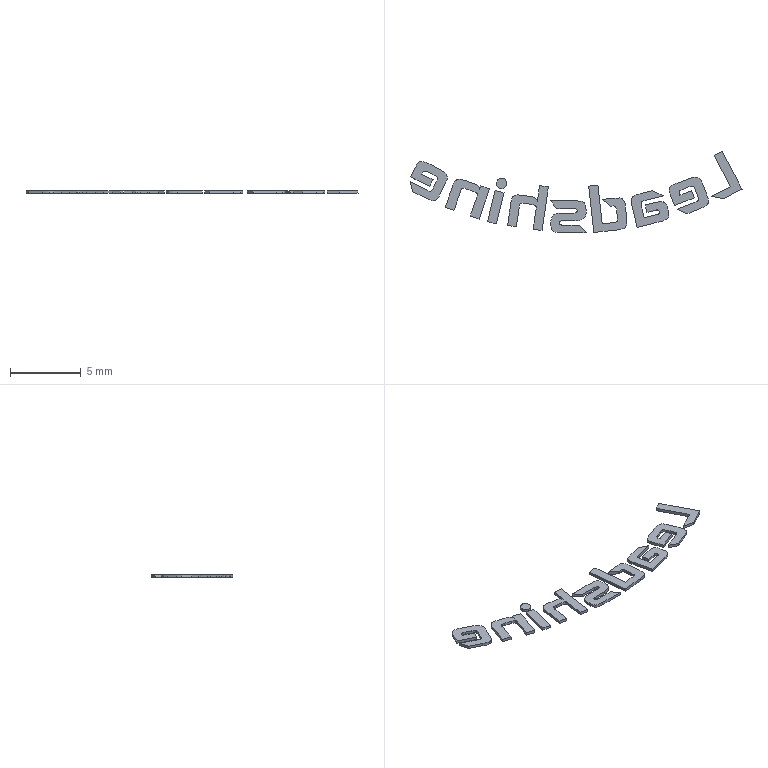Part | STEP file | LOGO123_1 | 10 solids | 180 faces | box 23.395 x 5.753 x 0.2 mm | volume 6.476 mm3 | plane 103 | spline 77